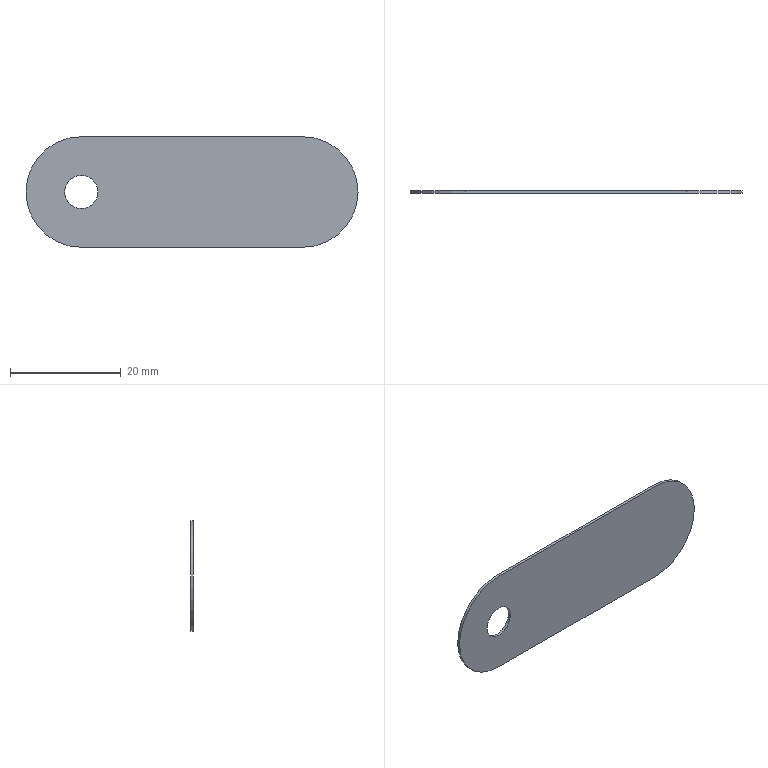Part | 1 solid | 8 faces | box 60 x 0.5 x 20 mm | volume 542.942 mm3 | cylinder 4 | plane 4 | commonest cylinder face diameters 6 x2 20 x2
STEP:
#1=CARTESIAN_POINT('',(0.,0.5,-3.));
#2=VERTEX_POINT('',#1);
#3=CARTESIAN_POINT('',(0.,0.5,3.));
#4=VERTEX_POINT('',#3);
#5=CARTESIAN_POINT('',(0.,0.5,0.));
#6=DIRECTION('',(0.,1.,0.));
#7=DIRECTION('',(0.,0.,1.));
#8=AXIS2_PLACEMENT_3D('',#5,#6,#7);
#9=CIRCLE('',#8,3.);
#10=EDGE_CURVE('',#2,#4,#9,.T.);
#11=ORIENTED_EDGE('',*,*,#10,.T.);
#12=CARTESIAN_POINT('',(0.,0.,3.));
#13=VERTEX_POINT('',#12);
#14=CARTESIAN_POINT('',(0.,0.5,3.));
#15=DIRECTION('',(0.,-1.,0.));
#16=VECTOR('',#15,1000.);
#17=LINE('',#14,#16);
#18=EDGE_CURVE('',#4,#13,#17,.T.);
#19=ORIENTED_EDGE('',*,*,#18,.T.);
#20=CARTESIAN_POINT('',(0.,0.,-3.));
#21=VERTEX_POINT('',#20);
#22=CARTESIAN_POINT('',(0.,0.,0.));
#23=DIRECTION('',(0.,1.,0.));
#24=DIRECTION('',(0.,0.,1.));
#25=AXIS2_PLACEMENT_3D('',#22,#23,#24);
#26=CIRCLE('',#25,3.);
#27=EDGE_CURVE('',#21,#13,#26,.T.);
#28=ORIENTED_EDGE('',*,*,#27,.F.);
#29=CARTESIAN_POINT('',(0.,0.5,-3.));
#30=DIRECTION('',(0.,-1.,0.));
#31=VECTOR('',#30,1000.);
#32=LINE('',#29,#31);
#33=EDGE_CURVE('',#2,#21,#32,.T.);
#34=ORIENTED_EDGE('',*,*,#33,.F.);
#35=EDGE_LOOP('',(#11,#19,#28,#34));
#36=FACE_OUTER_BOUND('',#35,.T.);
#37=CARTESIAN_POINT('',(0.,0.5,0.));
#38=DIRECTION('',(0.,-1.,0.));
#39=DIRECTION('',(0.,0.,-1.));
#40=AXIS2_PLACEMENT_3D('',#37,#38,#39);
#41=CYLINDRICAL_SURFACE('',#40,3.);
#42=ADVANCED_FACE('',(#36),#41,.F.);
#43=CARTESIAN_POINT('',(0.,0.5,-10.));
#44=VERTEX_POINT('',#43);
#45=CARTESIAN_POINT('',(0.,0.5,10.));
#46=VERTEX_POINT('',#45);
#47=CARTESIAN_POINT('',(0.,0.5,0.));
#48=DIRECTION('',(0.,1.,0.));
#49=DIRECTION('',(0.,0.,1.));
#50=AXIS2_PLACEMENT_3D('',#47,#48,#49);
#51=CIRCLE('',#50,10.);
#52=EDGE_CURVE('',#44,#46,#51,.T.);
#53=ORIENTED_EDGE('',*,*,#52,.T.);
#54=CARTESIAN_POINT('',(40.,0.5,10.));
#55=VERTEX_POINT('',#54);
#56=CARTESIAN_POINT('',(0.,0.5,10.));
#57=DIRECTION('',(1.,0.,0.));
#58=VECTOR('',#57,1000.);
#59=LINE('',#56,#58);
#60=EDGE_CURVE('',#46,#55,#59,.T.);
#61=ORIENTED_EDGE('',*,*,#60,.T.);
#62=CARTESIAN_POINT('',(40.,0.5,-10.));
#63=VERTEX_POINT('',#62);
#64=CARTESIAN_POINT('',(40.,0.5,0.));
#65=DIRECTION('',(0.,1.,0.));
#66=DIRECTION('',(0.,0.,1.));
#67=AXIS2_PLACEMENT_3D('',#64,#65,#66);
#68=CIRCLE('',#67,10.);
#69=EDGE_CURVE('',#55,#63,#68,.T.);
#70=ORIENTED_EDGE('',*,*,#69,.T.);
#71=CARTESIAN_POINT('',(0.,0.5,-10.));
#72=DIRECTION('',(-1.,0.,0.));
#73=VECTOR('',#72,1000.);
#74=LINE('',#71,#73);
#75=EDGE_CURVE('',#63,#44,#74,.T.);
#76=ORIENTED_EDGE('',*,*,#75,.T.);
#77=EDGE_LOOP('',(#53,#61,#70,#76));
#78=FACE_OUTER_BOUND('',#77,.T.);
#79=ORIENTED_EDGE('',*,*,#10,.F.);
#80=CARTESIAN_POINT('',(0.,0.5,0.));
#81=DIRECTION('',(0.,1.,0.));
#82=DIRECTION('',(0.,0.,1.));
#83=AXIS2_PLACEMENT_3D('',#80,#81,#82);
#84=CIRCLE('',#83,3.);
#85=EDGE_CURVE('',#4,#2,#84,.T.);
#86=ORIENTED_EDGE('',*,*,#85,.F.);
#87=EDGE_LOOP('',(#79,#86));
#88=FACE_BOUND('',#87,.T.);
#89=CARTESIAN_POINT('',(0.,0.5,0.));
#90=DIRECTION('',(0.,1.,0.));
#91=DIRECTION('',(0.,0.,1.));
#92=AXIS2_PLACEMENT_3D('',#89,#90,#91);
#93=PLANE('',#92);
#94=ADVANCED_FACE('',(#78,#88),#93,.T.);
#95=CARTESIAN_POINT('',(0.,0.,-10.));
#96=VERTEX_POINT('',#95);
#97=CARTESIAN_POINT('',(0.,0.,10.));
#98=VERTEX_POINT('',#97);
#99=CARTESIAN_POINT('',(0.,0.,0.));
#100=DIRECTION('',(0.,1.,0.));
#101=DIRECTION('',(0.,0.,1.));
#102=AXIS2_PLACEMENT_3D('',#99,#100,#101);
#103=CIRCLE('',#102,10.);
#104=EDGE_CURVE('',#96,#98,#103,.T.);
#105=ORIENTED_EDGE('',*,*,#104,.F.);
#106=CARTESIAN_POINT('',(40.,0.,-10.));
#107=VERTEX_POINT('',#106);
#108=CARTESIAN_POINT('',(0.,0.,-10.));
#109=DIRECTION('',(-1.,0.,0.));
#110=VECTOR('',#109,1000.);
#111=LINE('',#108,#110);
#112=EDGE_CURVE('',#107,#96,#111,.T.);
#113=ORIENTED_EDGE('',*,*,#112,.F.);
#114=CARTESIAN_POINT('',(40.,0.,10.));
#115=VERTEX_POINT('',#114);
#116=CARTESIAN_POINT('',(40.,0.,0.));
#117=DIRECTION('',(0.,1.,0.));
#118=DIRECTION('',(0.,0.,1.));
#119=AXIS2_PLACEMENT_3D('',#116,#117,#118);
#120=CIRCLE('',#119,10.);
#121=EDGE_CURVE('',#115,#107,#120,.T.);
#122=ORIENTED_EDGE('',*,*,#121,.F.);
#123=CARTESIAN_POINT('',(0.,0.,10.));
#124=DIRECTION('',(1.,0.,0.));
#125=VECTOR('',#124,1000.);
#126=LINE('',#123,#125);
#127=EDGE_CURVE('',#98,#115,#126,.T.);
#128=ORIENTED_EDGE('',*,*,#127,.F.);
#129=EDGE_LOOP('',(#105,#113,#122,#128));
#130=FACE_OUTER_BOUND('',#129,.T.);
#131=ORIENTED_EDGE('',*,*,#27,.T.);
#132=CARTESIAN_POINT('',(0.,0.,0.));
#133=DIRECTION('',(0.,1.,0.));
#134=DIRECTION('',(0.,0.,1.));
#135=AXIS2_PLACEMENT_3D('',#132,#133,#134);
#136=CIRCLE('',#135,3.);
#137=EDGE_CURVE('',#13,#21,#136,.T.);
#138=ORIENTED_EDGE('',*,*,#137,.T.);
#139=EDGE_LOOP('',(#131,#138));
#140=FACE_BOUND('',#139,.T.);
#141=CARTESIAN_POINT('',(0.,0.,0.));
#142=DIRECTION('',(0.,1.,0.));
#143=DIRECTION('',(0.,0.,1.));
#144=AXIS2_PLACEMENT_3D('',#141,#142,#143);
#145=PLANE('',#144);
#146=ADVANCED_FACE('',(#130,#140),#145,.F.);
#147=ORIENTED_EDGE('',*,*,#104,.T.);
#148=CARTESIAN_POINT('',(0.,0.5,10.));
#149=DIRECTION('',(0.,-1.,0.));
#150=VECTOR('',#149,1000.);
#151=LINE('',#148,#150);
#152=EDGE_CURVE('',#46,#98,#151,.T.);
#153=ORIENTED_EDGE('',*,*,#152,.F.);
#154=ORIENTED_EDGE('',*,*,#52,.F.);
#155=CARTESIAN_POINT('',(0.,0.5,-10.));
#156=DIRECTION('',(0.,-1.,0.));
#157=VECTOR('',#156,1000.);
#158=LINE('',#155,#157);
#159=EDGE_CURVE('',#44,#96,#158,.T.);
#160=ORIENTED_EDGE('',*,*,#159,.T.);
#161=EDGE_LOOP('',(#147,#153,#154,#160));
#162=FACE_OUTER_BOUND('',#161,.T.);
#163=CARTESIAN_POINT('',(0.,0.5,0.));
#164=DIRECTION('',(0.,-1.,0.));
#165=DIRECTION('',(0.,0.,-1.));
#166=AXIS2_PLACEMENT_3D('',#163,#164,#165);
#167=CYLINDRICAL_SURFACE('',#166,10.);
#168=ADVANCED_FACE('',(#162),#167,.T.);
#169=ORIENTED_EDGE('',*,*,#127,.T.);
#170=CARTESIAN_POINT('',(40.,0.5,10.));
#171=DIRECTION('',(0.,-1.,0.));
#172=VECTOR('',#171,1000.);
#173=LINE('',#170,#172);
#174=EDGE_CURVE('',#55,#115,#173,.T.);
#175=ORIENTED_EDGE('',*,*,#174,.F.);
#176=ORIENTED_EDGE('',*,*,#60,.F.);
#177=ORIENTED_EDGE('',*,*,#152,.T.);
#178=EDGE_LOOP('',(#169,#175,#176,#177));
#179=FACE_OUTER_BOUND('',#178,.T.);
#180=CARTESIAN_POINT('',(0.,0.5,10.));
#181=DIRECTION('',(0.,0.,-1.));
#182=DIRECTION('',(-1.,0.,0.));
#183=AXIS2_PLACEMENT_3D('',#180,#181,#182);
#184=PLANE('',#183);
#185=ADVANCED_FACE('',(#179),#184,.F.);
#186=ORIENTED_EDGE('',*,*,#121,.T.);
#187=CARTESIAN_POINT('',(40.,0.5,-10.));
#188=DIRECTION('',(0.,-1.,0.));
#189=VECTOR('',#188,1000.);
#190=LINE('',#187,#189);
#191=EDGE_CURVE('',#63,#107,#190,.T.);
#192=ORIENTED_EDGE('',*,*,#191,.F.);
#193=ORIENTED_EDGE('',*,*,#69,.F.);
#194=ORIENTED_EDGE('',*,*,#174,.T.);
#195=EDGE_LOOP('',(#186,#192,#193,#194));
#196=FACE_OUTER_BOUND('',#195,.T.);
#197=CARTESIAN_POINT('',(40.,0.5,0.));
#198=DIRECTION('',(0.,-1.,0.));
#199=DIRECTION('',(0.,0.,-1.));
#200=AXIS2_PLACEMENT_3D('',#197,#198,#199);
#201=CYLINDRICAL_SURFACE('',#200,10.);
#202=ADVANCED_FACE('',(#196),#201,.T.);
#203=ORIENTED_EDGE('',*,*,#112,.T.);
#204=ORIENTED_EDGE('',*,*,#159,.F.);
#205=ORIENTED_EDGE('',*,*,#75,.F.);
#206=ORIENTED_EDGE('',*,*,#191,.T.);
#207=EDGE_LOOP('',(#203,#204,#205,#206));
#208=FACE_OUTER_BOUND('',#207,.T.);
#209=CARTESIAN_POINT('',(0.,0.5,-10.));
#210=DIRECTION('',(0.,0.,1.));
#211=DIRECTION('',(1.,0.,0.));
#212=AXIS2_PLACEMENT_3D('',#209,#210,#211);
#213=PLANE('',#212);
#214=ADVANCED_FACE('',(#208),#213,.F.);
#215=ORIENTED_EDGE('',*,*,#18,.F.);
#216=ORIENTED_EDGE('',*,*,#85,.T.);
#217=ORIENTED_EDGE('',*,*,#33,.T.);
#218=ORIENTED_EDGE('',*,*,#137,.F.);
#219=EDGE_LOOP('',(#215,#216,#217,#218));
#220=FACE_OUTER_BOUND('',#219,.T.);
#221=CARTESIAN_POINT('',(0.,0.5,0.));
#222=DIRECTION('',(0.,-1.,0.));
#223=DIRECTION('',(0.,0.,-1.));
#224=AXIS2_PLACEMENT_3D('',#221,#222,#223);
#225=CYLINDRICAL_SURFACE('',#224,3.);
#226=ADVANCED_FACE('',(#220),#225,.F.);
#227=CLOSED_SHELL('',(#42,#94,#146,#168,#185,#202,#214,#226));
#228=MANIFOLD_SOLID_BREP('',#227);
#229=CARTESIAN_POINT('',(0.,0.,0.));
#230=DIRECTION('',(0.,0.,1.));
#231=DIRECTION('',(1.,0.,0.));
#232=AXIS2_PLACEMENT_3D('',#229,#230,#231);
#233=(LENGTH_UNIT()NAMED_UNIT(*)SI_UNIT(.MILLI.,.METRE.));
#234=UNCERTAINTY_MEASURE_WITH_UNIT(LENGTH_MEASURE(0.00001),#233,'','');
#235=(NAMED_UNIT(*)PLANE_ANGLE_UNIT()SI_UNIT($,.RADIAN.));
#236=(NAMED_UNIT(*)SI_UNIT($,.STERADIAN.)SOLID_ANGLE_UNIT());
#237=(GEOMETRIC_REPRESENTATION_CONTEXT(3)GLOBAL_UNCERTAINTY_ASSIGNED_CONTEXT((#234))GLOBAL_UNIT_ASSIGNED_CONTEXT((#233,#235,#236))REPRESENTATION_CONTEXT('',''));
#238=ADVANCED_BREP_SHAPE_REPRESENTATION('',(#228,#232),#237);